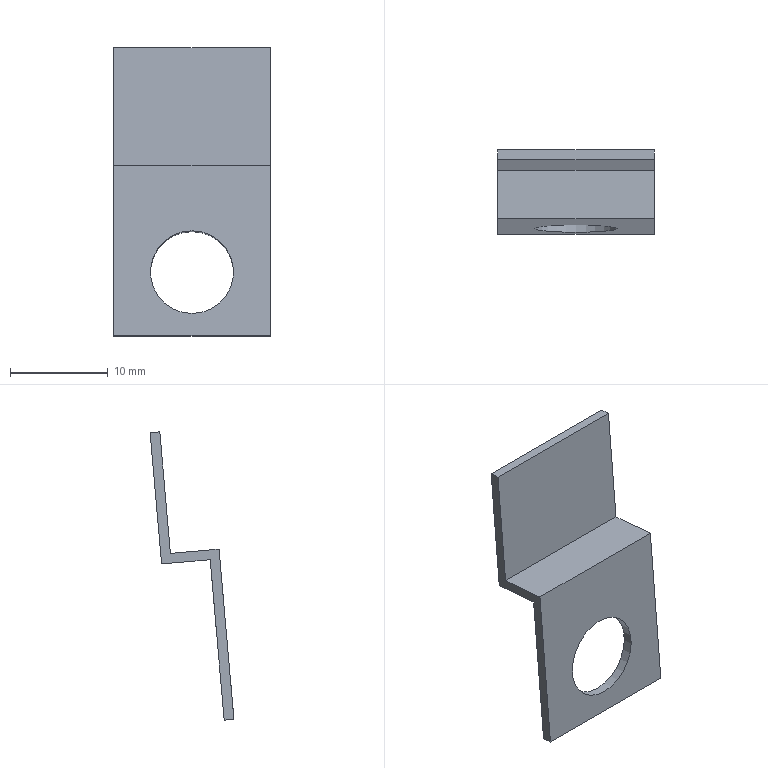Part | NX | features solid 2 | 1 solid | 11 faces | box 16 x 8.592 x 29.537 mm | volume 503.255 mm3 | plane 10 | cylinder 1 | commonest cylinder face diameters 8.5 x1
STEP:
#1=CARTESIAN_POINT('',(272.775,-116.761,-63.298));
#2=VERTEX_POINT('',#1);
#3=CARTESIAN_POINT('',(288.775,-116.761,-63.298));
#4=VERTEX_POINT('',#3);
#5=CARTESIAN_POINT('',(272.775,-116.761,-63.298));
#6=DIRECTION('',(1.,0.,0.));
#7=VECTOR('',#6,1000.);
#8=LINE('',#5,#7);
#9=EDGE_CURVE('',#2,#4,#8,.T.);
#10=ORIENTED_EDGE('',*,*,#9,.F.);
#11=CARTESIAN_POINT('',(272.775,-118.287,-80.731));
#12=VERTEX_POINT('',#11);
#13=CARTESIAN_POINT('',(272.775,-116.848,-64.294));
#14=DIRECTION('',(0.,0.08716,0.9962));
#15=VECTOR('',#14,1000.);
#16=LINE('',#13,#15);
#17=EDGE_CURVE('',#12,#2,#16,.T.);
#18=ORIENTED_EDGE('',*,*,#17,.F.);
#19=CARTESIAN_POINT('',(288.775,-118.287,-80.731));
#20=VERTEX_POINT('',#19);
#21=CARTESIAN_POINT('',(272.775,-118.287,-80.731));
#22=DIRECTION('',(1.,0.,0.));
#23=VECTOR('',#22,1000.);
#24=LINE('',#21,#23);
#25=EDGE_CURVE('',#12,#20,#24,.T.);
#26=ORIENTED_EDGE('',*,*,#25,.T.);
#27=CARTESIAN_POINT('',(288.775,-116.761,-63.298));
#28=DIRECTION('',(0.,-0.08716,-0.9962));
#29=VECTOR('',#28,1000.);
#30=LINE('',#27,#29);
#31=EDGE_CURVE('',#4,#20,#30,.T.);
#32=ORIENTED_EDGE('',*,*,#31,.F.);
#33=EDGE_LOOP('',(#10,#18,#26,#32));
#34=FACE_BOUND('',#33,.T.);
#35=CARTESIAN_POINT('',(280.775,-118.09,-78.49));
#36=VERTEX_POINT('',#35);
#37=CARTESIAN_POINT('',(280.775,-117.72,-74.256));
#38=DIRECTION('',(0.,0.9962,-0.08716));
#39=DIRECTION('',(0.,-0.08716,-0.9962));
#40=AXIS2_PLACEMENT_3D('',#37,#38,#39);
#41=CIRCLE('',#40,4.25);
#42=EDGE_CURVE('',#36,#36,#41,.T.);
#43=ORIENTED_EDGE('',*,*,#42,.T.);
#44=EDGE_LOOP('',(#43));
#45=FACE_BOUND('',#44,.T.);
#46=CARTESIAN_POINT('',(288.775,-116.761,-63.298));
#47=DIRECTION('',(0.,0.9962,-0.08716));
#48=DIRECTION('',(0.,-0.08716,-0.9962));
#49=AXIS2_PLACEMENT_3D('',#46,#47,#48);
#50=PLANE('',#49);
#51=ADVANCED_FACE('',(#34,#45),#50,.F.);
#52=CARTESIAN_POINT('',(272.775,-117.29,-80.819));
#53=VERTEX_POINT('',#52);
#54=CARTESIAN_POINT('',(288.775,-117.29,-80.819));
#55=VERTEX_POINT('',#54);
#56=CARTESIAN_POINT('',(272.775,-117.29,-80.819));
#57=DIRECTION('',(1.,0.,0.));
#58=VECTOR('',#57,1000.);
#59=LINE('',#56,#58);
#60=EDGE_CURVE('',#53,#55,#59,.T.);
#61=ORIENTED_EDGE('',*,*,#60,.F.);
#62=CARTESIAN_POINT('',(272.775,-115.852,-64.381));
#63=VERTEX_POINT('',#62);
#64=CARTESIAN_POINT('',(272.775,-115.852,-64.381));
#65=DIRECTION('',(0.,-0.08716,-0.9962));
#66=VECTOR('',#65,1000.);
#67=LINE('',#64,#66);
#68=EDGE_CURVE('',#63,#53,#67,.T.);
#69=ORIENTED_EDGE('',*,*,#68,.F.);
#70=CARTESIAN_POINT('',(288.775,-115.852,-64.381));
#71=VERTEX_POINT('',#70);
#72=CARTESIAN_POINT('',(272.775,-115.852,-64.381));
#73=DIRECTION('',(1.,0.,0.));
#74=VECTOR('',#73,1000.);
#75=LINE('',#72,#74);
#76=EDGE_CURVE('',#63,#71,#75,.T.);
#77=ORIENTED_EDGE('',*,*,#76,.T.);
#78=CARTESIAN_POINT('',(288.775,-117.29,-80.819));
#79=DIRECTION('',(0.,0.08716,0.9962));
#80=VECTOR('',#79,1000.);
#81=LINE('',#78,#80);
#82=EDGE_CURVE('',#55,#71,#81,.T.);
#83=ORIENTED_EDGE('',*,*,#82,.F.);
#84=EDGE_LOOP('',(#61,#69,#77,#83));
#85=FACE_BOUND('',#84,.T.);
#86=CARTESIAN_POINT('',(280.775,-117.094,-78.577));
#87=VERTEX_POINT('',#86);
#88=CARTESIAN_POINT('',(280.775,-116.724,-74.343));
#89=DIRECTION('',(0.,0.9962,-0.08716));
#90=DIRECTION('',(0.,-0.08716,-0.9962));
#91=AXIS2_PLACEMENT_3D('',#88,#89,#90);
#92=CIRCLE('',#91,4.25);
#93=EDGE_CURVE('',#87,#87,#92,.T.);
#94=ORIENTED_EDGE('',*,*,#93,.F.);
#95=EDGE_LOOP('',(#94));
#96=FACE_BOUND('',#95,.T.);
#97=CARTESIAN_POINT('',(288.775,-117.29,-80.819));
#98=DIRECTION('',(0.,-0.9962,0.08716));
#99=DIRECTION('',(0.,0.08716,0.9962));
#100=AXIS2_PLACEMENT_3D('',#97,#98,#99);
#101=PLANE('',#100);
#102=ADVANCED_FACE('',(#85,#96),#101,.F.);
#103=CARTESIAN_POINT('',(288.775,-110.691,-51.281));
#104=VERTEX_POINT('',#103);
#105=CARTESIAN_POINT('',(272.775,-110.691,-51.281));
#106=VERTEX_POINT('',#105);
#107=CARTESIAN_POINT('',(288.775,-110.691,-51.281));
#108=DIRECTION('',(-1.,0.,0.));
#109=VECTOR('',#108,1000.);
#110=LINE('',#107,#109);
#111=EDGE_CURVE('',#104,#106,#110,.T.);
#112=ORIENTED_EDGE('',*,*,#111,.F.);
#113=CARTESIAN_POINT('',(288.775,-109.695,-51.368));
#114=VERTEX_POINT('',#113);
#115=CARTESIAN_POINT('',(288.775,-109.695,-51.368));
#116=DIRECTION('',(0.,-0.9962,0.08716));
#117=VECTOR('',#116,1000.);
#118=LINE('',#115,#117);
#119=EDGE_CURVE('',#114,#104,#118,.T.);
#120=ORIENTED_EDGE('',*,*,#119,.F.);
#121=CARTESIAN_POINT('',(272.775,-109.695,-51.368));
#122=VERTEX_POINT('',#121);
#123=CARTESIAN_POINT('',(288.775,-109.695,-51.368));
#124=DIRECTION('',(-1.,0.,0.));
#125=VECTOR('',#124,1000.);
#126=LINE('',#123,#125);
#127=EDGE_CURVE('',#114,#122,#126,.T.);
#128=ORIENTED_EDGE('',*,*,#127,.T.);
#129=CARTESIAN_POINT('',(272.775,-109.695,-51.368));
#130=DIRECTION('',(0.,-0.9962,0.08716));
#131=VECTOR('',#130,1000.);
#132=LINE('',#129,#131);
#133=EDGE_CURVE('',#122,#106,#132,.T.);
#134=ORIENTED_EDGE('',*,*,#133,.T.);
#135=EDGE_LOOP('',(#112,#120,#128,#134));
#136=FACE_BOUND('',#135,.T.);
#137=CARTESIAN_POINT('',(288.775,-109.695,-51.368));
#138=DIRECTION('',(0.,0.08716,0.9962));
#139=DIRECTION('',(0.,0.9962,-0.08716));
#140=AXIS2_PLACEMENT_3D('',#137,#138,#139);
#141=PLANE('',#140);
#142=ADVANCED_FACE('',(#136),#141,.T.);
#143=CARTESIAN_POINT('',(272.775,-111.78,-63.734));
#144=VERTEX_POINT('',#143);
#145=CARTESIAN_POINT('',(272.775,-110.691,-51.281));
#146=DIRECTION('',(0.,-0.08716,-0.9962));
#147=VECTOR('',#146,1000.);
#148=LINE('',#145,#147);
#149=EDGE_CURVE('',#106,#144,#148,.T.);
#150=ORIENTED_EDGE('',*,*,#149,.F.);
#151=ORIENTED_EDGE('',*,*,#133,.F.);
#152=CARTESIAN_POINT('',(272.775,-110.871,-64.817));
#153=VERTEX_POINT('',#152);
#154=CARTESIAN_POINT('',(272.775,-109.695,-51.368));
#155=DIRECTION('',(0.,-0.08716,-0.9962));
#156=VECTOR('',#155,1000.);
#157=LINE('',#154,#156);
#158=EDGE_CURVE('',#122,#153,#157,.T.);
#159=ORIENTED_EDGE('',*,*,#158,.T.);
#160=CARTESIAN_POINT('',(272.775,-110.871,-64.817));
#161=DIRECTION('',(0.,-0.9962,0.08716));
#162=VECTOR('',#161,1000.);
#163=LINE('',#160,#162);
#164=EDGE_CURVE('',#153,#63,#163,.T.);
#165=ORIENTED_EDGE('',*,*,#164,.T.);
#166=ORIENTED_EDGE('',*,*,#68,.T.);
#167=CARTESIAN_POINT('',(272.775,-117.29,-80.819));
#168=DIRECTION('',(0.,-0.9962,0.08716));
#169=VECTOR('',#168,1000.);
#170=LINE('',#167,#169);
#171=EDGE_CURVE('',#53,#12,#170,.T.);
#172=ORIENTED_EDGE('',*,*,#171,.T.);
#173=ORIENTED_EDGE('',*,*,#17,.T.);
#174=CARTESIAN_POINT('',(272.775,-110.784,-63.821));
#175=DIRECTION('',(0.,-0.9962,0.08716));
#176=VECTOR('',#175,1000.);
#177=LINE('',#174,#176);
#178=EDGE_CURVE('',#144,#2,#177,.T.);
#179=ORIENTED_EDGE('',*,*,#178,.F.);
#180=EDGE_LOOP('',(#150,#151,#159,#165,#166,#172,#173,#179));
#181=FACE_BOUND('',#180,.T.);
#182=CARTESIAN_POINT('',(272.775,-109.695,-51.368));
#183=DIRECTION('',(-1.,0.,0.));
#184=DIRECTION('',(0.,0.9962,-0.08716));
#185=AXIS2_PLACEMENT_3D('',#182,#183,#184);
#186=PLANE('',#185);
#187=ADVANCED_FACE('',(#181),#186,.T.);
#188=CARTESIAN_POINT('',(288.775,-111.78,-63.734));
#189=VERTEX_POINT('',#188);
#190=CARTESIAN_POINT('',(288.775,-111.78,-63.734));
#191=DIRECTION('',(0.,0.08716,0.9962));
#192=VECTOR('',#191,1000.);
#193=LINE('',#190,#192);
#194=EDGE_CURVE('',#189,#104,#193,.T.);
#195=ORIENTED_EDGE('',*,*,#194,.F.);
#196=CARTESIAN_POINT('',(288.775,-110.784,-63.821));
#197=DIRECTION('',(0.,-0.9962,0.08716));
#198=VECTOR('',#197,1000.);
#199=LINE('',#196,#198);
#200=EDGE_CURVE('',#189,#4,#199,.T.);
#201=ORIENTED_EDGE('',*,*,#200,.T.);
#202=ORIENTED_EDGE('',*,*,#31,.T.);
#203=CARTESIAN_POINT('',(288.775,-117.29,-80.819));
#204=DIRECTION('',(0.,-0.9962,0.08716));
#205=VECTOR('',#204,1000.);
#206=LINE('',#203,#205);
#207=EDGE_CURVE('',#55,#20,#206,.T.);
#208=ORIENTED_EDGE('',*,*,#207,.F.);
#209=ORIENTED_EDGE('',*,*,#82,.T.);
#210=CARTESIAN_POINT('',(288.775,-110.871,-64.817));
#211=VERTEX_POINT('',#210);
#212=CARTESIAN_POINT('',(288.775,-110.871,-64.817));
#213=DIRECTION('',(0.,-0.9962,0.08716));
#214=VECTOR('',#213,1000.);
#215=LINE('',#212,#214);
#216=EDGE_CURVE('',#211,#71,#215,.T.);
#217=ORIENTED_EDGE('',*,*,#216,.F.);
#218=CARTESIAN_POINT('',(288.775,-110.784,-63.821));
#219=DIRECTION('',(0.,0.08716,0.9962));
#220=VECTOR('',#219,1000.);
#221=LINE('',#218,#220);
#222=EDGE_CURVE('',#211,#114,#221,.T.);
#223=ORIENTED_EDGE('',*,*,#222,.T.);
#224=ORIENTED_EDGE('',*,*,#119,.T.);
#225=EDGE_LOOP('',(#195,#201,#202,#208,#209,#217,#223,#224));
#226=FACE_BOUND('',#225,.T.);
#227=CARTESIAN_POINT('',(288.775,-110.784,-63.821));
#228=DIRECTION('',(1.,0.,0.));
#229=DIRECTION('',(0.,-0.9962,0.08716));
#230=AXIS2_PLACEMENT_3D('',#227,#228,#229);
#231=PLANE('',#230);
#232=ADVANCED_FACE('',(#226),#231,.T.);
#233=ORIENTED_EDGE('',*,*,#127,.F.);
#234=ORIENTED_EDGE('',*,*,#222,.F.);
#235=CARTESIAN_POINT('',(272.775,-110.871,-64.817));
#236=DIRECTION('',(1.,0.,0.));
#237=VECTOR('',#236,1000.);
#238=LINE('',#235,#237);
#239=EDGE_CURVE('',#153,#211,#238,.T.);
#240=ORIENTED_EDGE('',*,*,#239,.F.);
#241=ORIENTED_EDGE('',*,*,#158,.F.);
#242=EDGE_LOOP('',(#233,#234,#240,#241));
#243=FACE_BOUND('',#242,.T.);
#244=CARTESIAN_POINT('',(272.775,-109.695,-51.368));
#245=DIRECTION('',(0.,-0.9962,0.08716));
#246=DIRECTION('',(0.,0.08716,0.9962));
#247=AXIS2_PLACEMENT_3D('',#244,#245,#246);
#248=PLANE('',#247);
#249=ADVANCED_FACE('',(#243),#248,.F.);
#250=ORIENTED_EDGE('',*,*,#111,.T.);
#251=ORIENTED_EDGE('',*,*,#149,.T.);
#252=CARTESIAN_POINT('',(272.775,-111.78,-63.734));
#253=DIRECTION('',(1.,0.,0.));
#254=VECTOR('',#253,1000.);
#255=LINE('',#252,#254);
#256=EDGE_CURVE('',#144,#189,#255,.T.);
#257=ORIENTED_EDGE('',*,*,#256,.T.);
#258=ORIENTED_EDGE('',*,*,#194,.T.);
#259=EDGE_LOOP('',(#250,#251,#257,#258));
#260=FACE_BOUND('',#259,.T.);
#261=CARTESIAN_POINT('',(272.775,-110.691,-51.281));
#262=DIRECTION('',(0.,-0.9962,0.08716));
#263=DIRECTION('',(0.,0.08716,0.9962));
#264=AXIS2_PLACEMENT_3D('',#261,#262,#263);
#265=PLANE('',#264);
#266=ADVANCED_FACE('',(#260),#265,.T.);
#267=ORIENTED_EDGE('',*,*,#256,.F.);
#268=ORIENTED_EDGE('',*,*,#178,.T.);
#269=ORIENTED_EDGE('',*,*,#9,.T.);
#270=ORIENTED_EDGE('',*,*,#200,.F.);
#271=EDGE_LOOP('',(#267,#268,#269,#270));
#272=FACE_BOUND('',#271,.T.);
#273=CARTESIAN_POINT('',(272.775,-110.784,-63.821));
#274=DIRECTION('',(0.,-0.08716,-0.9962));
#275=DIRECTION('',(0.,-0.9962,0.08716));
#276=AXIS2_PLACEMENT_3D('',#273,#274,#275);
#277=PLANE('',#276);
#278=ADVANCED_FACE('',(#272),#277,.F.);
#279=ORIENTED_EDGE('',*,*,#76,.F.);
#280=ORIENTED_EDGE('',*,*,#164,.F.);
#281=ORIENTED_EDGE('',*,*,#239,.T.);
#282=ORIENTED_EDGE('',*,*,#216,.T.);
#283=EDGE_LOOP('',(#279,#280,#281,#282));
#284=FACE_BOUND('',#283,.T.);
#285=CARTESIAN_POINT('',(272.775,-110.871,-64.817));
#286=DIRECTION('',(0.,-0.08716,-0.9962));
#287=DIRECTION('',(0.,-0.9962,0.08716));
#288=AXIS2_PLACEMENT_3D('',#285,#286,#287);
#289=PLANE('',#288);
#290=ADVANCED_FACE('',(#284),#289,.T.);
#291=ORIENTED_EDGE('',*,*,#25,.F.);
#292=ORIENTED_EDGE('',*,*,#171,.F.);
#293=ORIENTED_EDGE('',*,*,#60,.T.);
#294=ORIENTED_EDGE('',*,*,#207,.T.);
#295=EDGE_LOOP('',(#291,#292,#293,#294));
#296=FACE_BOUND('',#295,.T.);
#297=CARTESIAN_POINT('',(272.775,-117.29,-80.819));
#298=DIRECTION('',(0.,-0.08716,-0.9962));
#299=DIRECTION('',(0.,-0.9962,0.08716));
#300=AXIS2_PLACEMENT_3D('',#297,#298,#299);
#301=PLANE('',#300);
#302=ADVANCED_FACE('',(#296),#301,.T.);
#303=ORIENTED_EDGE('',*,*,#93,.T.);
#304=EDGE_LOOP('',(#303));
#305=FACE_BOUND('',#304,.T.);
#306=ORIENTED_EDGE('',*,*,#42,.F.);
#307=EDGE_LOOP('',(#306));
#308=FACE_BOUND('',#307,.T.);
#309=CARTESIAN_POINT('',(280.775,-116.724,-74.343));
#310=DIRECTION('',(0.,-0.9962,0.08716));
#311=DIRECTION('',(0.,0.08716,0.9962));
#312=AXIS2_PLACEMENT_3D('',#309,#310,#311);
#313=CYLINDRICAL_SURFACE('',#312,4.25);
#314=ADVANCED_FACE('',(#305,#308),#313,.F.);
#315=CLOSED_SHELL('',(#51,#102,#142,#187,#232,#249,#266,#278,#290,#302,#314));
#316=MANIFOLD_SOLID_BREP('',#315);
#317=(LENGTH_UNIT()NAMED_UNIT(*)SI_UNIT(.MILLI.,.METRE.));
#318=UNCERTAINTY_MEASURE_WITH_UNIT(LENGTH_MEASURE(0.00001),#317,'','');
#319=(NAMED_UNIT(*)PLANE_ANGLE_UNIT()SI_UNIT($,.RADIAN.));
#320=(NAMED_UNIT(*)SI_UNIT($,.STERADIAN.)SOLID_ANGLE_UNIT());
#321=(GEOMETRIC_REPRESENTATION_CONTEXT(3)GLOBAL_UNCERTAINTY_ASSIGNED_CONTEXT((#318))GLOBAL_UNIT_ASSIGNED_CONTEXT((#317,#319,#320))REPRESENTATION_CONTEXT('',''));
#322=ADVANCED_BREP_SHAPE_REPRESENTATION('',(#316),#321);